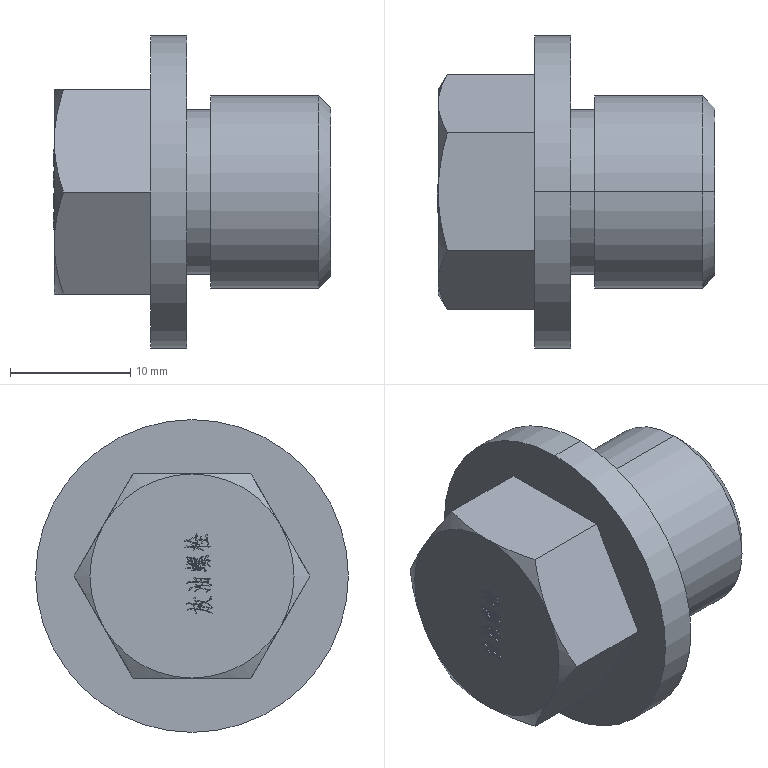Part | SolidWorks | features Chamfer 1, Extrusion 1, ICE 1, RevCut 1, Revolution 1 | 1 solid | 544 faces | box 23.1 x 26 x 26 mm | volume 5865 mm3 | plane 412 | spline 118 | cone 8 | cylinder 6 | commonest cylinder face diameters 13.7 x2 16 x2 26 x2